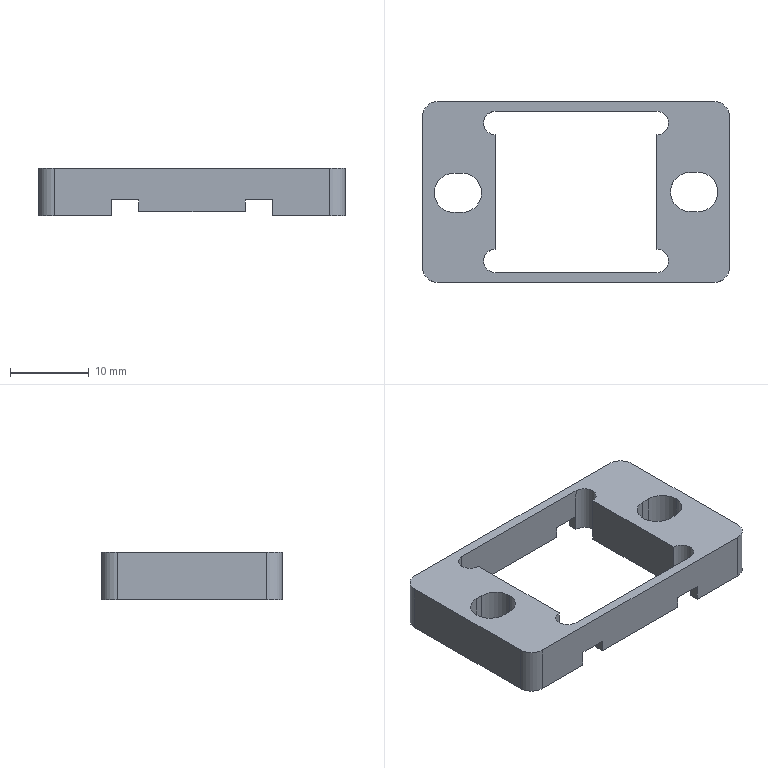Part | SolidWorks | features ICE 4, Cut 1, Extrusion 1, Fillet 1 | 1 solid | 45 faces | box 39 x 23 x 6 mm | volume 2408 mm3 | plane 29 | cylinder 16 | commonest cylinder face diameters 3 x6 5 x6 4 x4
STEP:
#1=CARTESIAN_POINT('',(-12.,-0.1,0.));
#2=VERTEX_POINT('',#1);
#3=CARTESIAN_POINT('',(-14.5,2.4,0.));
#4=VERTEX_POINT('',#3);
#5=CARTESIAN_POINT('',(-14.5,-0.1,0.));
#6=DIRECTION('',(0.,0.,1.));
#7=DIRECTION('',(1.,0.,0.));
#8=AXIS2_PLACEMENT_3D('',#5,#6,#7);
#9=CIRCLE('',#8,2.5);
#10=EDGE_CURVE('',#2,#4,#9,.T.);
#11=ORIENTED_EDGE('',*,*,#10,.F.);
#12=CARTESIAN_POINT('',(-12.,-0.1,6.));
#13=VERTEX_POINT('',#12);
#14=CARTESIAN_POINT('',(-12.,-0.1,-4.));
#15=DIRECTION('',(0.,0.,1.));
#16=VECTOR('',#15,1000.);
#17=LINE('',#14,#16);
#18=EDGE_CURVE('',#2,#13,#17,.T.);
#19=ORIENTED_EDGE('',*,*,#18,.T.);
#20=CARTESIAN_POINT('',(-14.5,2.4,6.));
#21=VERTEX_POINT('',#20);
#22=CARTESIAN_POINT('',(-14.5,-0.1,6.));
#23=DIRECTION('',(0.,0.,1.));
#24=DIRECTION('',(1.,0.,0.));
#25=AXIS2_PLACEMENT_3D('',#22,#23,#24);
#26=CIRCLE('',#25,2.5);
#27=EDGE_CURVE('',#13,#21,#26,.T.);
#28=ORIENTED_EDGE('',*,*,#27,.T.);
#29=CARTESIAN_POINT('',(-14.5,2.4,-4.));
#30=DIRECTION('',(0.,0.,1.));
#31=VECTOR('',#30,1000.);
#32=LINE('',#29,#31);
#33=EDGE_CURVE('',#4,#21,#32,.T.);
#34=ORIENTED_EDGE('',*,*,#33,.F.);
#35=EDGE_LOOP('',(#11,#19,#28,#34));
#36=FACE_OUTER_BOUND('',#35,.T.);
#37=CARTESIAN_POINT('',(-14.5,-0.1,-4.));
#38=DIRECTION('',(0.,0.,1.));
#39=DIRECTION('',(1.,0.,0.));
#40=AXIS2_PLACEMENT_3D('',#37,#38,#39);
#41=CYLINDRICAL_SURFACE('',#40,2.5);
#42=ADVANCED_FACE('',(#36),#41,.F.);
#43=CARTESIAN_POINT('',(18.,0.,0.));
#44=VERTEX_POINT('',#43);
#45=CARTESIAN_POINT('',(15.5,2.5,0.));
#46=VERTEX_POINT('',#45);
#47=CARTESIAN_POINT('',(15.5,0.,0.));
#48=DIRECTION('',(0.,0.,1.));
#49=DIRECTION('',(1.,0.,0.));
#50=AXIS2_PLACEMENT_3D('',#47,#48,#49);
#51=CIRCLE('',#50,2.5);
#52=EDGE_CURVE('',#44,#46,#51,.T.);
#53=ORIENTED_EDGE('',*,*,#52,.F.);
#54=CARTESIAN_POINT('',(18.,0.,6.));
#55=VERTEX_POINT('',#54);
#56=CARTESIAN_POINT('',(18.,0.,-4.));
#57=DIRECTION('',(0.,0.,1.));
#58=VECTOR('',#57,1000.);
#59=LINE('',#56,#58);
#60=EDGE_CURVE('',#44,#55,#59,.T.);
#61=ORIENTED_EDGE('',*,*,#60,.T.);
#62=CARTESIAN_POINT('',(15.5,2.5,6.));
#63=VERTEX_POINT('',#62);
#64=CARTESIAN_POINT('',(15.5,0.,6.));
#65=DIRECTION('',(0.,0.,1.));
#66=DIRECTION('',(1.,0.,0.));
#67=AXIS2_PLACEMENT_3D('',#64,#65,#66);
#68=CIRCLE('',#67,2.5);
#69=EDGE_CURVE('',#55,#63,#68,.T.);
#70=ORIENTED_EDGE('',*,*,#69,.T.);
#71=CARTESIAN_POINT('',(15.5,2.5,-4.));
#72=DIRECTION('',(0.,0.,1.));
#73=VECTOR('',#72,1000.);
#74=LINE('',#71,#73);
#75=EDGE_CURVE('',#46,#63,#74,.T.);
#76=ORIENTED_EDGE('',*,*,#75,.F.);
#77=EDGE_LOOP('',(#53,#61,#70,#76));
#78=FACE_OUTER_BOUND('',#77,.T.);
#79=CARTESIAN_POINT('',(15.5,0.,-4.));
#80=DIRECTION('',(0.,0.,1.));
#81=DIRECTION('',(1.,0.,0.));
#82=AXIS2_PLACEMENT_3D('',#79,#80,#81);
#83=CYLINDRICAL_SURFACE('',#82,2.5);
#84=ADVANCED_FACE('',(#78),#83,.F.);
#85=CARTESIAN_POINT('',(-11.75,8.75,6.));
#86=VERTEX_POINT('',#85);
#87=CARTESIAN_POINT('',(-10.25,10.25,6.));
#88=VERTEX_POINT('',#87);
#89=CARTESIAN_POINT('',(-10.25,8.75,6.));
#90=DIRECTION('',(0.,0.,-1.));
#91=DIRECTION('',(1.,0.,0.));
#92=AXIS2_PLACEMENT_3D('',#89,#90,#91);
#93=CIRCLE('',#92,1.5);
#94=EDGE_CURVE('',#86,#88,#93,.T.);
#95=ORIENTED_EDGE('',*,*,#94,.F.);
#96=CARTESIAN_POINT('',(-11.75,8.75,0.));
#97=VERTEX_POINT('',#96);
#98=CARTESIAN_POINT('',(-11.75,8.75,29.691));
#99=DIRECTION('',(0.,0.,-1.));
#100=VECTOR('',#99,1000.);
#101=LINE('',#98,#100);
#102=EDGE_CURVE('',#86,#97,#101,.T.);
#103=ORIENTED_EDGE('',*,*,#102,.T.);
#104=CARTESIAN_POINT('',(-10.25,10.25,0.));
#105=VERTEX_POINT('',#104);
#106=CARTESIAN_POINT('',(-10.25,8.75,0.));
#107=DIRECTION('',(0.,0.,-1.));
#108=DIRECTION('',(-1.,0.,0.));
#109=AXIS2_PLACEMENT_3D('',#106,#107,#108);
#110=CIRCLE('',#109,1.5);
#111=EDGE_CURVE('',#97,#105,#110,.T.);
#112=ORIENTED_EDGE('',*,*,#111,.T.);
#113=CARTESIAN_POINT('',(-10.25,10.25,2.));
#114=VERTEX_POINT('',#113);
#115=CARTESIAN_POINT('',(-10.25,10.25,29.691));
#116=DIRECTION('',(0.,0.,-1.));
#117=VECTOR('',#116,1000.);
#118=LINE('',#115,#117);
#119=EDGE_CURVE('',#114,#105,#118,.T.);
#120=ORIENTED_EDGE('',*,*,#119,.F.);
#121=CARTESIAN_POINT('',(-10.25,10.25,6.));
#122=DIRECTION('',(0.,0.,-1.));
#123=VECTOR('',#122,1000.);
#124=LINE('',#121,#123);
#125=EDGE_CURVE('',#88,#114,#124,.T.);
#126=ORIENTED_EDGE('',*,*,#125,.F.);
#127=EDGE_LOOP('',(#95,#103,#112,#120,#126));
#128=FACE_OUTER_BOUND('',#127,.T.);
#129=CARTESIAN_POINT('',(-10.25,8.75,29.691));
#130=DIRECTION('',(0.,0.,-1.));
#131=DIRECTION('',(-1.,0.,0.));
#132=AXIS2_PLACEMENT_3D('',#129,#130,#131);
#133=CYLINDRICAL_SURFACE('',#132,1.5);
#134=ADVANCED_FACE('',(#128),#133,.F.);
#135=CARTESIAN_POINT('',(-11.75,-8.75,6.));
#136=VERTEX_POINT('',#135);
#137=CARTESIAN_POINT('',(-10.25,-7.25,6.));
#138=VERTEX_POINT('',#137);
#139=CARTESIAN_POINT('',(-10.25,-8.75,6.));
#140=DIRECTION('',(0.,0.,-1.));
#141=DIRECTION('',(1.,0.,0.));
#142=AXIS2_PLACEMENT_3D('',#139,#140,#141);
#143=CIRCLE('',#142,1.5);
#144=EDGE_CURVE('',#136,#138,#143,.T.);
#145=ORIENTED_EDGE('',*,*,#144,.F.);
#146=CARTESIAN_POINT('',(-11.75,-8.75,0.));
#147=VERTEX_POINT('',#146);
#148=CARTESIAN_POINT('',(-11.75,-8.75,29.691));
#149=DIRECTION('',(0.,0.,-1.));
#150=VECTOR('',#149,1000.);
#151=LINE('',#148,#150);
#152=EDGE_CURVE('',#136,#147,#151,.T.);
#153=ORIENTED_EDGE('',*,*,#152,.T.);
#154=CARTESIAN_POINT('',(-10.25,-7.25,0.));
#155=VERTEX_POINT('',#154);
#156=CARTESIAN_POINT('',(-10.25,-8.75,0.));
#157=DIRECTION('',(0.,0.,-1.));
#158=DIRECTION('',(-1.,0.,0.));
#159=AXIS2_PLACEMENT_3D('',#156,#157,#158);
#160=CIRCLE('',#159,1.5);
#161=EDGE_CURVE('',#147,#155,#160,.T.);
#162=ORIENTED_EDGE('',*,*,#161,.T.);
#163=CARTESIAN_POINT('',(-10.25,-7.25,29.691));
#164=DIRECTION('',(0.,0.,-1.));
#165=VECTOR('',#164,1000.);
#166=LINE('',#163,#165);
#167=EDGE_CURVE('',#138,#155,#166,.T.);
#168=ORIENTED_EDGE('',*,*,#167,.F.);
#169=EDGE_LOOP('',(#145,#153,#162,#168));
#170=FACE_OUTER_BOUND('',#169,.T.);
#171=CARTESIAN_POINT('',(-10.25,-8.75,29.691));
#172=DIRECTION('',(0.,0.,-1.));
#173=DIRECTION('',(-1.,0.,0.));
#174=AXIS2_PLACEMENT_3D('',#171,#172,#173);
#175=CYLINDRICAL_SURFACE('',#174,1.5);
#176=ADVANCED_FACE('',(#170),#175,.F.);
#177=CARTESIAN_POINT('',(10.25,10.25,2.));
#178=VERTEX_POINT('',#177);
#179=CARTESIAN_POINT('',(10.25,10.25,0.));
#180=VERTEX_POINT('',#179);
#181=CARTESIAN_POINT('',(10.25,10.25,29.691));
#182=DIRECTION('',(0.,0.,-1.));
#183=VECTOR('',#182,1000.);
#184=LINE('',#181,#183);
#185=EDGE_CURVE('',#178,#180,#184,.T.);
#186=ORIENTED_EDGE('',*,*,#185,.F.);
#187=CARTESIAN_POINT('',(10.25,11.5,2.));
#188=VERTEX_POINT('',#187);
#189=CARTESIAN_POINT('',(10.25,32.097,2.));
#190=DIRECTION('',(0.,-1.,0.));
#191=VECTOR('',#190,1000.);
#192=LINE('',#189,#191);
#193=EDGE_CURVE('',#188,#178,#192,.T.);
#194=ORIENTED_EDGE('',*,*,#193,.F.);
#195=CARTESIAN_POINT('',(10.25,11.5,0.));
#196=VERTEX_POINT('',#195);
#197=CARTESIAN_POINT('',(10.25,11.5,0.));
#198=DIRECTION('',(0.,0.,-1.));
#199=VECTOR('',#198,1000.);
#200=LINE('',#197,#199);
#201=EDGE_CURVE('',#188,#196,#200,.T.);
#202=ORIENTED_EDGE('',*,*,#201,.T.);
#203=CARTESIAN_POINT('',(10.25,10.25,0.));
#204=DIRECTION('',(0.,1.,0.));
#205=VECTOR('',#204,1000.);
#206=LINE('',#203,#205);
#207=EDGE_CURVE('',#180,#196,#206,.T.);
#208=ORIENTED_EDGE('',*,*,#207,.F.);
#209=EDGE_LOOP('',(#186,#194,#202,#208));
#210=FACE_OUTER_BOUND('',#209,.T.);
#211=CARTESIAN_POINT('',(10.25,10.25,6.));
#212=DIRECTION('',(-1.,0.,0.));
#213=DIRECTION('',(0.,-1.,0.));
#214=AXIS2_PLACEMENT_3D('',#211,#212,#213);
#215=PLANE('',#214);
#216=ADVANCED_FACE('',(#210),#215,.T.);
#217=CARTESIAN_POINT('',(10.25,7.25,6.));
#218=VERTEX_POINT('',#217);
#219=CARTESIAN_POINT('',(10.25,7.25,0.));
#220=VERTEX_POINT('',#219);
#221=CARTESIAN_POINT('',(10.25,7.25,29.691));
#222=DIRECTION('',(0.,0.,-1.));
#223=VECTOR('',#222,1000.);
#224=LINE('',#221,#223);
#225=EDGE_CURVE('',#218,#220,#224,.T.);
#226=ORIENTED_EDGE('',*,*,#225,.T.);
#227=CARTESIAN_POINT('',(10.25,-7.25,0.));
#228=VERTEX_POINT('',#227);
#229=CARTESIAN_POINT('',(10.25,10.25,0.));
#230=DIRECTION('',(0.,1.,0.));
#231=VECTOR('',#230,1000.);
#232=LINE('',#229,#231);
#233=EDGE_CURVE('',#228,#220,#232,.T.);
#234=ORIENTED_EDGE('',*,*,#233,.F.);
#235=CARTESIAN_POINT('',(10.25,-7.25,6.));
#236=VERTEX_POINT('',#235);
#237=CARTESIAN_POINT('',(10.25,-7.25,29.691));
#238=DIRECTION('',(0.,0.,-1.));
#239=VECTOR('',#238,1000.);
#240=LINE('',#237,#239);
#241=EDGE_CURVE('',#236,#228,#240,.T.);
#242=ORIENTED_EDGE('',*,*,#241,.F.);
#243=CARTESIAN_POINT('',(10.25,10.25,6.));
#244=DIRECTION('',(0.,1.,0.));
#245=VECTOR('',#244,1000.);
#246=LINE('',#243,#245);
#247=EDGE_CURVE('',#236,#218,#246,.T.);
#248=ORIENTED_EDGE('',*,*,#247,.T.);
#249=EDGE_LOOP('',(#226,#234,#242,#248));
#250=FACE_OUTER_BOUND('',#249,.T.);
#251=CARTESIAN_POINT('',(10.25,10.25,6.));
#252=DIRECTION('',(-1.,0.,0.));
#253=DIRECTION('',(0.,-1.,0.));
#254=AXIS2_PLACEMENT_3D('',#251,#252,#253);
#255=PLANE('',#254);
#256=ADVANCED_FACE('',(#250),#255,.T.);
#257=CARTESIAN_POINT('',(-10.25,7.25,6.));
#258=VERTEX_POINT('',#257);
#259=CARTESIAN_POINT('',(-10.25,7.25,0.));
#260=VERTEX_POINT('',#259);
#261=CARTESIAN_POINT('',(-10.25,7.25,29.691));
#262=DIRECTION('',(0.,0.,-1.));
#263=VECTOR('',#262,1000.);
#264=LINE('',#261,#263);
#265=EDGE_CURVE('',#258,#260,#264,.T.);
#266=ORIENTED_EDGE('',*,*,#265,.F.);
#267=CARTESIAN_POINT('',(-10.25,10.25,6.));
#268=DIRECTION('',(0.,-1.,0.));
#269=VECTOR('',#268,1000.);
#270=LINE('',#267,#269);
#271=EDGE_CURVE('',#258,#138,#270,.T.);
#272=ORIENTED_EDGE('',*,*,#271,.T.);
#273=ORIENTED_EDGE('',*,*,#167,.T.);
#274=CARTESIAN_POINT('',(-10.25,10.25,0.));
#275=DIRECTION('',(0.,-1.,0.));
#276=VECTOR('',#275,1000.);
#277=LINE('',#274,#276);
#278=EDGE_CURVE('',#260,#155,#277,.T.);
#279=ORIENTED_EDGE('',*,*,#278,.F.);
#280=EDGE_LOOP('',(#266,#272,#273,#279));
#281=FACE_OUTER_BOUND('',#280,.T.);
#282=CARTESIAN_POINT('',(-10.25,10.25,6.));
#283=DIRECTION('',(1.,0.,0.));
#284=DIRECTION('',(0.,1.,0.));
#285=AXIS2_PLACEMENT_3D('',#282,#283,#284);
#286=PLANE('',#285);
#287=ADVANCED_FACE('',(#281),#286,.T.);
#288=CARTESIAN_POINT('',(-10.25,-10.25,2.));
#289=VERTEX_POINT('',#288);
#290=CARTESIAN_POINT('',(-10.25,-10.25,0.));
#291=VERTEX_POINT('',#290);
#292=CARTESIAN_POINT('',(-10.25,-10.25,29.691));
#293=DIRECTION('',(0.,0.,-1.));
#294=VECTOR('',#293,1000.);
#295=LINE('',#292,#294);
#296=EDGE_CURVE('',#289,#291,#295,.T.);
#297=ORIENTED_EDGE('',*,*,#296,.F.);
#298=CARTESIAN_POINT('',(-10.25,-11.5,2.));
#299=VERTEX_POINT('',#298);
#300=CARTESIAN_POINT('',(-10.25,32.097,2.));
#301=DIRECTION('',(0.,-1.,0.));
#302=VECTOR('',#301,1000.);
#303=LINE('',#300,#302);
#304=EDGE_CURVE('',#289,#299,#303,.T.);
#305=ORIENTED_EDGE('',*,*,#304,.T.);
#306=CARTESIAN_POINT('',(-10.25,-11.5,0.));
#307=VERTEX_POINT('',#306);
#308=CARTESIAN_POINT('',(-10.25,-11.5,0.));
#309=DIRECTION('',(0.,0.,-1.));
#310=VECTOR('',#309,1000.);
#311=LINE('',#308,#310);
#312=EDGE_CURVE('',#299,#307,#311,.T.);
#313=ORIENTED_EDGE('',*,*,#312,.T.);
#314=CARTESIAN_POINT('',(-10.25,10.25,0.));
#315=DIRECTION('',(0.,-1.,0.));
#316=VECTOR('',#315,1000.);
#317=LINE('',#314,#316);
#318=EDGE_CURVE('',#291,#307,#317,.T.);
#319=ORIENTED_EDGE('',*,*,#318,.F.);
#320=EDGE_LOOP('',(#297,#305,#313,#319));
#321=FACE_OUTER_BOUND('',#320,.T.);
#322=CARTESIAN_POINT('',(-10.25,10.25,6.));
#323=DIRECTION('',(1.,0.,0.));
#324=DIRECTION('',(0.,1.,0.));
#325=AXIS2_PLACEMENT_3D('',#322,#323,#324);
#326=PLANE('',#325);
#327=ADVANCED_FACE('',(#321),#326,.T.);
#328=CARTESIAN_POINT('',(-15.5,2.4,0.));
#329=VERTEX_POINT('',#328);
#330=CARTESIAN_POINT('',(0.,2.4,0.));
#331=DIRECTION('',(-1.,0.,0.));
#332=VECTOR('',#331,1000.);
#333=LINE('',#330,#332);
#334=EDGE_CURVE('',#4,#329,#333,.T.);
#335=ORIENTED_EDGE('',*,*,#334,.T.);
#336=CARTESIAN_POINT('',(-15.5,-2.6,0.));
#337=VERTEX_POINT('',#336);
#338=CARTESIAN_POINT('',(-15.5,-0.1,0.));
#339=DIRECTION('',(0.,0.,1.));
#340=DIRECTION('',(1.,0.,0.));
#341=AXIS2_PLACEMENT_3D('',#338,#339,#340);
#342=CIRCLE('',#341,2.5);
#343=EDGE_CURVE('',#329,#337,#342,.T.);
#344=ORIENTED_EDGE('',*,*,#343,.T.);
#345=CARTESIAN_POINT('',(-14.5,-2.6,0.));
#346=VERTEX_POINT('',#345);
#347=CARTESIAN_POINT('',(0.,-2.6,0.));
#348=DIRECTION('',(1.,0.,0.));
#349=VECTOR('',#348,1000.);
#350=LINE('',#347,#349);
#351=EDGE_CURVE('',#337,#346,#350,.T.);
#352=ORIENTED_EDGE('',*,*,#351,.T.);
#353=CARTESIAN_POINT('',(-14.5,-0.1,0.));
#354=DIRECTION('',(0.,0.,1.));
#355=DIRECTION('',(1.,0.,0.));
#356=AXIS2_PLACEMENT_3D('',#353,#354,#355);
#357=CIRCLE('',#356,2.5);
#358=EDGE_CURVE('',#346,#2,#357,.T.);
#359=ORIENTED_EDGE('',*,*,#358,.T.);
#360=ORIENTED_EDGE('',*,*,#10,.T.);
#361=EDGE_LOOP('',(#335,#344,#352,#359,#360));
#362=FACE_BOUND('',#361,.T.);
#363=CARTESIAN_POINT('',(-19.5,9.5,0.));
#364=VERTEX_POINT('',#363);
#365=CARTESIAN_POINT('',(-19.5,-9.5,0.));
#366=VERTEX_POINT('',#365);
#367=CARTESIAN_POINT('',(-19.5,11.5,0.));
#368=DIRECTION('',(0.,-1.,0.));
#369=VECTOR('',#368,1000.);
#370=LINE('',#367,#369);
#371=EDGE_CURVE('',#364,#366,#370,.T.);
#372=ORIENTED_EDGE('',*,*,#371,.F.);
#373=CARTESIAN_POINT('',(-17.5,11.5,0.));
#374=VERTEX_POINT('',#373);
#375=CARTESIAN_POINT('',(-17.5,9.5,0.));
#376=DIRECTION('',(0.,0.,-1.));
#377=DIRECTION('',(1.,0.,0.));
#378=AXIS2_PLACEMENT_3D('',#375,#376,#377);
#379=CIRCLE('',#378,2.);
#380=EDGE_CURVE('',#364,#374,#379,.T.);
#381=ORIENTED_EDGE('',*,*,#380,.T.);
#382=CARTESIAN_POINT('',(-10.25,11.5,0.));
#383=VERTEX_POINT('',#382);
#384=CARTESIAN_POINT('',(-19.5,11.5,0.));
#385=DIRECTION('',(-1.,0.,0.));
#386=VECTOR('',#385,1000.);
#387=LINE('',#384,#386);
#388=EDGE_CURVE('',#383,#374,#387,.T.);
#389=ORIENTED_EDGE('',*,*,#388,.F.);
#390=CARTESIAN_POINT('',(-10.25,10.25,0.));
#391=DIRECTION('',(0.,-1.,0.));
#392=VECTOR('',#391,1000.);
#393=LINE('',#390,#392);
#394=EDGE_CURVE('',#383,#105,#393,.T.);
#395=ORIENTED_EDGE('',*,*,#394,.T.);
#396=ORIENTED_EDGE('',*,*,#111,.F.);
#397=CARTESIAN_POINT('',(-10.25,8.75,0.));
#398=DIRECTION('',(0.,0.,-1.));
#399=DIRECTION('',(-1.,0.,0.));
#400=AXIS2_PLACEMENT_3D('',#397,#398,#399);
#401=CIRCLE('',#400,1.5);
#402=EDGE_CURVE('',#260,#97,#401,.T.);
#403=ORIENTED_EDGE('',*,*,#402,.F.);
#404=ORIENTED_EDGE('',*,*,#278,.T.);
#405=ORIENTED_EDGE('',*,*,#161,.F.);
#406=CARTESIAN_POINT('',(-10.25,-8.75,0.));
#407=DIRECTION('',(0.,0.,-1.));
#408=DIRECTION('',(-1.,0.,0.));
#409=AXIS2_PLACEMENT_3D('',#406,#407,#408);
#410=CIRCLE('',#409,1.5);
#411=EDGE_CURVE('',#291,#147,#410,.T.);
#412=ORIENTED_EDGE('',*,*,#411,.F.);
#413=ORIENTED_EDGE('',*,*,#318,.T.);
#414=CARTESIAN_POINT('',(-17.5,-11.5,0.));
#415=VERTEX_POINT('',#414);
#416=CARTESIAN_POINT('',(-19.5,-11.5,0.));
#417=DIRECTION('',(1.,0.,0.));
#418=VECTOR('',#417,1000.);
#419=LINE('',#416,#418);
#420=EDGE_CURVE('',#415,#307,#419,.T.);
#421=ORIENTED_EDGE('',*,*,#420,.F.);
#422=CARTESIAN_POINT('',(-17.5,-9.5,0.));
#423=DIRECTION('',(0.,0.,-1.));
#424=DIRECTION('',(1.,0.,0.));
#425=AXIS2_PLACEMENT_3D('',#422,#423,#424);
#426=CIRCLE('',#425,2.);
#427=EDGE_CURVE('',#415,#366,#426,.T.);
#428=ORIENTED_EDGE('',*,*,#427,.T.);
#429=EDGE_LOOP('',(#372,#381,#389,#395,#396,#403,#404,#405,#412,#413,#421,#428));
#430=FACE_OUTER_BOUND('',#429,.T.);
#431=CARTESIAN_POINT('',(0.,0.,0.));
#432=DIRECTION('',(0.,0.,1.));
#433=DIRECTION('',(1.,0.,0.));
#434=AXIS2_PLACEMENT_3D('',#431,#432,#433);
#435=PLANE('',#434);
#436=ADVANCED_FACE('',(#362,#430),#435,.F.);
#437=CARTESIAN_POINT('',(-15.5,2.4,6.));
#438=VERTEX_POINT('',#437);
#439=CARTESIAN_POINT('',(-15.5,-2.6,6.));
#440=VERTEX_POINT('',#439);
#441=CARTESIAN_POINT('',(-15.5,-0.1,6.));
#442=DIRECTION('',(0.,0.,1.));
#443=DIRECTION('',(1.,0.,0.));
#444=AXIS2_PLACEMENT_3D('',#441,#442,#443);
#445=CIRCLE('',#444,2.5);
#446=EDGE_CURVE('',#438,#440,#445,.T.);
#447=ORIENTED_EDGE('',*,*,#446,.F.);
#448=CARTESIAN_POINT('',(-15.5,2.4,6.));
#449=DIRECTION('',(-1.,0.,0.));
#450=VECTOR('',#449,1000.);
#451=LINE('',#448,#450);
#452=EDGE_CURVE('',#21,#438,#451,.T.);
#453=ORIENTED_EDGE('',*,*,#452,.F.);
#454=ORIENTED_EDGE('',*,*,#27,.F.);
#455=CARTESIAN_POINT('',(-14.5,-2.6,6.));
#456=VERTEX_POINT('',#455);
#457=CARTESIAN_POINT('',(-14.5,-0.1,6.));
#458=DIRECTION('',(0.,0.,1.));
#459=DIRECTION('',(1.,0.,0.));
#460=AXIS2_PLACEMENT_3D('',#457,#458,#459);
#461=CIRCLE('',#460,2.5);
#462=EDGE_CURVE('',#456,#13,#461,.T.);
#463=ORIENTED_EDGE('',*,*,#462,.F.);
#464=CARTESIAN_POINT('',(-15.5,-2.6,6.));
#465=DIRECTION('',(1.,0.,0.));
#466=VECTOR('',#465,1000.);
#467=LINE('',#464,#466);
#468=EDGE_CURVE('',#440,#456,#467,.T.);
#469=ORIENTED_EDGE('',*,*,#468,.F.);
#470=EDGE_LOOP('',(#447,#453,#454,#463,#469));
#471=FACE_BOUND('',#470,.T.);
#472=CARTESIAN_POINT('',(14.5,2.5,6.));
#473=VERTEX_POINT('',#472);
#474=CARTESIAN_POINT('',(14.5,-2.5,6.));
#475=VERTEX_POINT('',#474);
#476=CARTESIAN_POINT('',(14.5,0.,6.));
#477=DIRECTION('',(0.,0.,1.));
#478=DIRECTION('',(1.,0.,0.));
#479=AXIS2_PLACEMENT_3D('',#476,#477,#478);
#480=CIRCLE('',#479,2.5);
#481=EDGE_CURVE('',#473,#475,#480,.T.);
#482=ORIENTED_EDGE('',*,*,#481,.F.);
#483=CARTESIAN_POINT('',(14.5,2.5,6.));
#484=DIRECTION('',(-1.,0.,0.));
#485=VECTOR('',#484,1000.);
#486=LINE('',#483,#485);
#487=EDGE_CURVE('',#63,#473,#486,.T.);
#488=ORIENTED_EDGE('',*,*,#487,.F.);
#489=ORIENTED_EDGE('',*,*,#69,.F.);
#490=CARTESIAN_POINT('',(15.5,-2.5,6.));
#491=VERTEX_POINT('',#490);
#492=CARTESIAN_POINT('',(15.5,0.,6.));
#493=DIRECTION('',(0.,0.,1.));
#494=DIRECTION('',(1.,0.,0.));
#495=AXIS2_PLACEMENT_3D('',#492,#493,#494);
#496=CIRCLE('',#495,2.5);
#497=EDGE_CURVE('',#491,#55,#496,.T.);
#498=ORIENTED_EDGE('',*,*,#497,.F.);
#499=CARTESIAN_POINT('',(14.5,-2.5,6.));
#500=DIRECTION('',(1.,0.,0.));
#501=VECTOR('',#500,1000.);
#502=LINE('',#499,#501);
#503=EDGE_CURVE('',#475,#491,#502,.T.);
#504=ORIENTED_EDGE('',*,*,#503,.F.);
#505=EDGE_LOOP('',(#482,#488,#489,#498,#504));
#506=FACE_BOUND('',#505,.T.);
#507=CARTESIAN_POINT('',(-10.25,8.75,6.));
#508=DIRECTION('',(0.,0.,-1.));
#509=DIRECTION('',(1.,0.,0.));
#510=AXIS2_PLACEMENT_3D('',#507,#508,#509);
#511=CIRCLE('',#510,1.5);
#512=EDGE_CURVE('',#258,#86,#511,.T.);
#513=ORIENTED_EDGE('',*,*,#512,.T.);
#514=ORIENTED_EDGE('',*,*,#94,.T.);
#515=CARTESIAN_POINT('',(10.25,10.25,6.));
#516=VERTEX_POINT('',#515);
#517=CARTESIAN_POINT('',(-10.25,10.25,6.));
#518=DIRECTION('',(1.,0.,0.));
#519=VECTOR('',#518,1000.);
#520=LINE('',#517,#519);
#521=EDGE_CURVE('',#88,#516,#520,.T.);
#522=ORIENTED_EDGE('',*,*,#521,.T.);
#523=CARTESIAN_POINT('',(10.25,8.75,6.));
#524=DIRECTION('',(0.,0.,-1.));
#525=DIRECTION('',(1.,0.,0.));
#526=AXIS2_PLACEMENT_3D('',#523,#524,#525);
#527=CIRCLE('',#526,1.5);
#528=EDGE_CURVE('',#516,#218,#527,.T.);
#529=ORIENTED_EDGE('',*,*,#528,.T.);
#530=ORIENTED_EDGE('',*,*,#247,.F.);
#531=CARTESIAN_POINT('',(10.25,-10.25,6.));
#532=VERTEX_POINT('',#531);
#533=CARTESIAN_POINT('',(10.25,-8.75,6.));
#534=DIRECTION('',(0.,0.,-1.));
#535=DIRECTION('',(1.,0.,0.));
#536=AXIS2_PLACEMENT_3D('',#533,#534,#535);
#537=CIRCLE('',#536,1.5);
#538=EDGE_CURVE('',#236,#532,#537,.T.);
#539=ORIENTED_EDGE('',*,*,#538,.T.);
#540=CARTESIAN_POINT('',(-10.25,-10.25,6.));
#541=VERTEX_POINT('',#540);
#542=CARTESIAN_POINT('',(-10.25,-10.25,6.));
#543=DIRECTION('',(-1.,0.,0.));
#544=VECTOR('',#543,1000.);
#545=LINE('',#542,#544);
#546=EDGE_CURVE('',#532,#541,#545,.T.);
#547=ORIENTED_EDGE('',*,*,#546,.T.);
#548=CARTESIAN_POINT('',(-10.25,-8.75,6.));
#549=DIRECTION('',(0.,0.,-1.));
#550=DIRECTION('',(1.,0.,0.));
#551=AXIS2_PLACEMENT_3D('',#548,#549,#550);
#552=CIRCLE('',#551,1.5);
#553=EDGE_CURVE('',#541,#136,#552,.T.);
#554=ORIENTED_EDGE('',*,*,#553,.T.);
#555=ORIENTED_EDGE('',*,*,#144,.T.);
#556=ORIENTED_EDGE('',*,*,#271,.F.);
#557=EDGE_LOOP('',(#513,#514,#522,#529,#530,#539,#547,#554,#555,#556));
#558=FACE_BOUND('',#557,.T.);
#559=CARTESIAN_POINT('',(17.5,11.5,6.));
#560=VERTEX_POINT('',#559);
#561=CARTESIAN_POINT('',(-17.5,11.5,6.));
#562=VERTEX_POINT('',#561);
#563=CARTESIAN_POINT('',(-19.5,11.5,6.));
#564=DIRECTION('',(-1.,0.,0.));
#565=VECTOR('',#564,1000.);
#566=LINE('',#563,#565);
#567=EDGE_CURVE('',#560,#562,#566,.T.);
#568=ORIENTED_EDGE('',*,*,#567,.T.);
#569=CARTESIAN_POINT('',(-19.5,9.5,6.));
#570=VERTEX_POINT('',#569);
#571=CARTESIAN_POINT('',(-17.5,9.5,6.));
#572=DIRECTION('',(0.,0.,1.));
#573=DIRECTION('',(1.,0.,0.));
#574=AXIS2_PLACEMENT_3D('',#571,#572,#573);
#575=CIRCLE('',#574,2.);
#576=EDGE_CURVE('',#562,#570,#575,.T.);
#577=ORIENTED_EDGE('',*,*,#576,.T.);
#578=CARTESIAN_POINT('',(-19.5,-9.5,6.));
#579=VERTEX_POINT('',#578);
#580=CARTESIAN_POINT('',(-19.5,11.5,6.));
#581=DIRECTION('',(0.,-1.,0.));
#582=VECTOR('',#581,1000.);
#583=LINE('',#580,#582);
#584=EDGE_CURVE('',#570,#579,#583,.T.);
#585=ORIENTED_EDGE('',*,*,#584,.T.);
#586=CARTESIAN_POINT('',(-17.5,-11.5,6.));
#587=VERTEX_POINT('',#586);
#588=CARTESIAN_POINT('',(-17.5,-9.5,6.));
#589=DIRECTION('',(0.,0.,1.));
#590=DIRECTION('',(1.,0.,0.));
#591=AXIS2_PLACEMENT_3D('',#588,#589,#590);
#592=CIRCLE('',#591,2.);
#593=EDGE_CURVE('',#579,#587,#592,.T.);
#594=ORIENTED_EDGE('',*,*,#593,.T.);
#595=CARTESIAN_POINT('',(17.5,-11.5,6.));
#596=VERTEX_POINT('',#595);
#597=CARTESIAN_POINT('',(-19.5,-11.5,6.));
#598=DIRECTION('',(1.,0.,0.));
#599=VECTOR('',#598,1000.);
#600=LINE('',#597,#599);
#601=EDGE_CURVE('',#587,#596,#600,.T.);
#602=ORIENTED_EDGE('',*,*,#601,.T.);
#603=CARTESIAN_POINT('',(19.5,-9.5,6.));
#604=VERTEX_POINT('',#603);
#605=CARTESIAN_POINT('',(17.5,-9.5,6.));
#606=DIRECTION('',(0.,0.,1.));
#607=DIRECTION('',(1.,0.,0.));
#608=AXIS2_PLACEMENT_3D('',#605,#606,#607);
#609=CIRCLE('',#608,2.);
#610=EDGE_CURVE('',#596,#604,#609,.T.);
#611=ORIENTED_EDGE('',*,*,#610,.T.);
#612=CARTESIAN_POINT('',(19.5,9.5,6.));
#613=VERTEX_POINT('',#612);
#614=CARTESIAN_POINT('',(19.5,11.5,6.));
#615=DIRECTION('',(0.,1.,0.));
#616=VECTOR('',#615,1000.);
#617=LINE('',#614,#616);
#618=EDGE_CURVE('',#604,#613,#617,.T.);
#619=ORIENTED_EDGE('',*,*,#618,.T.);
#620=CARTESIAN_POINT('',(17.5,9.5,6.));
#621=DIRECTION('',(0.,0.,1.));
#622=DIRECTION('',(1.,0.,0.));
#623=AXIS2_PLACEMENT_3D('',#620,#621,#622);
#624=CIRCLE('',#623,2.);
#625=EDGE_CURVE('',#613,#560,#624,.T.);
#626=ORIENTED_EDGE('',*,*,#625,.T.);
#627=EDGE_LOOP('',(#568,#577,#585,#594,#602,#611,#619,#626));
#628=FACE_OUTER_BOUND('',#627,.T.);
#629=CARTESIAN_POINT('',(0.,0.,6.));
#630=DIRECTION('',(0.,0.,1.));
#631=DIRECTION('',(1.,0.,0.));
#632=AXIS2_PLACEMENT_3D('',#629,#630,#631);
#633=PLANE('',#632);
#634=ADVANCED_FACE('',(#471,#506,#558,#628),#633,.T.);
#635=CARTESIAN_POINT('',(14.5,2.5,0.));
#636=VERTEX_POINT('',#635);
#637=CARTESIAN_POINT('',(0.,2.5,0.));
#638=DIRECTION('',(-1.,0.,0.));
#639=VECTOR('',#638,1000.);
#640=LINE('',#637,#639);
#641=EDGE_CURVE('',#46,#636,#640,.T.);
#642=ORIENTED_EDGE('',*,*,#641,.T.);
#643=CARTESIAN_POINT('',(14.5,-2.5,0.));
#644=VERTEX_POINT('',#643);
#645=CARTESIAN_POINT('',(14.5,0.,0.));
#646=DIRECTION('',(0.,0.,1.));
#647=DIRECTION('',(1.,0.,0.));
#648=AXIS2_PLACEMENT_3D('',#645,#646,#647);
#649=CIRCLE('',#648,2.5);
#650=EDGE_CURVE('',#636,#644,#649,.T.);
#651=ORIENTED_EDGE('',*,*,#650,.T.);
#652=CARTESIAN_POINT('',(15.5,-2.5,0.));
#653=VERTEX_POINT('',#652);
#654=CARTESIAN_POINT('',(0.,-2.5,0.));
#655=DIRECTION('',(1.,0.,0.));
#656=VECTOR('',#655,1000.);
#657=LINE('',#654,#656);
#658=EDGE_CURVE('',#644,#653,#657,.T.);
#659=ORIENTED_EDGE('',*,*,#658,.T.);
#660=CARTESIAN_POINT('',(15.5,0.,0.));
#661=DIRECTION('',(0.,0.,1.));
#662=DIRECTION('',(1.,0.,0.));
#663=AXIS2_PLACEMENT_3D('',#660,#661,#662);
#664=CIRCLE('',#663,2.5);
#665=EDGE_CURVE('',#653,#44,#664,.T.);
#666=ORIENTED_EDGE('',*,*,#665,.T.);
#667=ORIENTED_EDGE('',*,*,#52,.T.);
#668=EDGE_LOOP('',(#642,#651,#659,#666,#667));
#669=FACE_BOUND('',#668,.T.);
#670=CARTESIAN_POINT('',(19.5,-9.5,0.));
#671=VERTEX_POINT('',#670);
#672=CARTESIAN_POINT('',(19.5,9.5,0.));
#673=VERTEX_POINT('',#672);
#674=CARTESIAN_POINT('',(19.5,11.5,0.));
#675=DIRECTION('',(0.,1.,0.));
#676=VECTOR('',#675,1000.);
#677=LINE('',#674,#676);
#678=EDGE_CURVE('',#671,#673,#677,.T.);
#679=ORIENTED_EDGE('',*,*,#678,.F.);
#680=CARTESIAN_POINT('',(17.5,-11.5,0.));
#681=VERTEX_POINT('',#680);
#682=CARTESIAN_POINT('',(17.5,-9.5,0.));
#683=DIRECTION('',(0.,0.,-1.));
#684=DIRECTION('',(1.,0.,0.));
#685=AXIS2_PLACEMENT_3D('',#682,#683,#684);
#686=CIRCLE('',#685,2.);
#687=EDGE_CURVE('',#671,#681,#686,.T.);
#688=ORIENTED_EDGE('',*,*,#687,.T.);
#689=CARTESIAN_POINT('',(10.25,-11.5,0.));
#690=VERTEX_POINT('',#689);
#691=CARTESIAN_POINT('',(-19.5,-11.5,0.));
#692=DIRECTION('',(1.,0.,0.));
#693=VECTOR('',#692,1000.);
#694=LINE('',#691,#693);
#695=EDGE_CURVE('',#690,#681,#694,.T.);
#696=ORIENTED_EDGE('',*,*,#695,.F.);
#697=CARTESIAN_POINT('',(10.25,-10.25,0.));
#698=VERTEX_POINT('',#697);
#699=CARTESIAN_POINT('',(10.25,10.25,0.));
#700=DIRECTION('',(0.,1.,0.));
#701=VECTOR('',#700,1000.);
#702=LINE('',#699,#701);
#703=EDGE_CURVE('',#690,#698,#702,.T.);
#704=ORIENTED_EDGE('',*,*,#703,.T.);
#705=CARTESIAN_POINT('',(10.25,-8.75,0.));
#706=DIRECTION('',(0.,0.,-1.));
#707=DIRECTION('',(-1.,0.,0.));
#708=AXIS2_PLACEMENT_3D('',#705,#706,#707);
#709=CIRCLE('',#708,1.5);
#710=EDGE_CURVE('',#228,#698,#709,.T.);
#711=ORIENTED_EDGE('',*,*,#710,.F.);
#712=ORIENTED_EDGE('',*,*,#233,.T.);
#713=CARTESIAN_POINT('',(10.25,8.75,0.));
#714=DIRECTION('',(0.,0.,-1.));
#715=DIRECTION('',(-1.,0.,0.));
#716=AXIS2_PLACEMENT_3D('',#713,#714,#715);
#717=CIRCLE('',#716,1.5);
#718=EDGE_CURVE('',#180,#220,#717,.T.);
#719=ORIENTED_EDGE('',*,*,#718,.F.);
#720=ORIENTED_EDGE('',*,*,#207,.T.);
#721=CARTESIAN_POINT('',(17.5,11.5,0.));
#722=VERTEX_POINT('',#721);
#723=CARTESIAN_POINT('',(-19.5,11.5,0.));
#724=DIRECTION('',(-1.,0.,0.));
#725=VECTOR('',#724,1000.);
#726=LINE('',#723,#725);
#727=EDGE_CURVE('',#722,#196,#726,.T.);
#728=ORIENTED_EDGE('',*,*,#727,.F.);
#729=CARTESIAN_POINT('',(17.5,9.5,0.));
#730=DIRECTION('',(0.,0.,-1.));
#731=DIRECTION('',(1.,0.,0.));
#732=AXIS2_PLACEMENT_3D('',#729,#730,#731);
#733=CIRCLE('',#732,2.);
#734=EDGE_CURVE('',#722,#673,#733,.T.);
#735=ORIENTED_EDGE('',*,*,#734,.T.);
#736=EDGE_LOOP('',(#679,#688,#696,#704,#711,#712,#719,#720,#728,#735));
#737=FACE_OUTER_BOUND('',#736,.T.);
#738=CARTESIAN_POINT('',(0.,0.,0.));
#739=DIRECTION('',(0.,0.,1.));
#740=DIRECTION('',(1.,0.,0.));
#741=AXIS2_PLACEMENT_3D('',#738,#739,#740);
#742=PLANE('',#741);
#743=ADVANCED_FACE('',(#669,#737),#742,.F.);
#744=ORIENTED_EDGE('',*,*,#618,.F.);
#745=CARTESIAN_POINT('',(19.5,-9.5,6.));
#746=DIRECTION('',(0.,0.,-1.));
#747=VECTOR('',#746,1000.);
#748=LINE('',#745,#747);
#749=EDGE_CURVE('',#604,#671,#748,.T.);
#750=ORIENTED_EDGE('',*,*,#749,.T.);
#751=ORIENTED_EDGE('',*,*,#678,.T.);
#752=CARTESIAN_POINT('',(19.5,9.5,6.));
#753=DIRECTION('',(0.,0.,1.));
#754=VECTOR('',#753,1000.);
#755=LINE('',#752,#754);
#756=EDGE_CURVE('',#673,#613,#755,.T.);
#757=ORIENTED_EDGE('',*,*,#756,.T.);
#758=EDGE_LOOP('',(#744,#750,#751,#757));
#759=FACE_OUTER_BOUND('',#758,.T.);
#760=CARTESIAN_POINT('',(19.5,11.5,6.));
#761=DIRECTION('',(-1.,0.,0.));
#762=DIRECTION('',(0.,-1.,0.));
#763=AXIS2_PLACEMENT_3D('',#760,#761,#762);
#764=PLANE('',#763);
#765=ADVANCED_FACE('',(#759),#764,.F.);
#766=ORIENTED_EDGE('',*,*,#388,.T.);
#767=CARTESIAN_POINT('',(-17.5,11.5,6.));
#768=DIRECTION('',(0.,0.,1.));
#769=VECTOR('',#768,1000.);
#770=LINE('',#767,#769);
#771=EDGE_CURVE('',#374,#562,#770,.T.);
#772=ORIENTED_EDGE('',*,*,#771,.T.);
#773=ORIENTED_EDGE('',*,*,#567,.F.);
#774=CARTESIAN_POINT('',(17.5,11.5,6.));
#775=DIRECTION('',(0.,0.,-1.));
#776=VECTOR('',#775,1000.);
#777=LINE('',#774,#776);
#778=EDGE_CURVE('',#560,#722,#777,.T.);
#779=ORIENTED_EDGE('',*,*,#778,.T.);
#780=ORIENTED_EDGE('',*,*,#727,.T.);
#781=ORIENTED_EDGE('',*,*,#201,.F.);
#782=CARTESIAN_POINT('',(6.75,11.5,2.));
#783=VERTEX_POINT('',#782);
#784=CARTESIAN_POINT('',(10.25,11.5,2.));
#785=DIRECTION('',(1.,0.,0.));
#786=VECTOR('',#785,1000.);
#787=LINE('',#784,#786);
#788=EDGE_CURVE('',#783,#188,#787,.T.);
#789=ORIENTED_EDGE('',*,*,#788,.F.);
#790=CARTESIAN_POINT('',(6.75,11.5,0.5));
#791=VERTEX_POINT('',#790);
#792=CARTESIAN_POINT('',(6.75,11.5,0.5));
#793=DIRECTION('',(0.,0.,1.));
#794=VECTOR('',#793,1000.);
#795=LINE('',#792,#794);
#796=EDGE_CURVE('',#791,#783,#795,.T.);
#797=ORIENTED_EDGE('',*,*,#796,.F.);
#798=CARTESIAN_POINT('',(-6.75,11.5,0.5));
#799=VERTEX_POINT('',#798);
#800=CARTESIAN_POINT('',(-6.75,11.5,0.5));
#801=DIRECTION('',(1.,0.,0.));
#802=VECTOR('',#801,1000.);
#803=LINE('',#800,#802);
#804=EDGE_CURVE('',#799,#791,#803,.T.);
#805=ORIENTED_EDGE('',*,*,#804,.F.);
#806=CARTESIAN_POINT('',(-6.75,11.5,2.));
#807=VERTEX_POINT('',#806);
#808=CARTESIAN_POINT('',(-6.75,11.5,0.5));
#809=DIRECTION('',(0.,0.,-1.));
#810=VECTOR('',#809,1000.);
#811=LINE('',#808,#810);
#812=EDGE_CURVE('',#807,#799,#811,.T.);
#813=ORIENTED_EDGE('',*,*,#812,.F.);
#814=CARTESIAN_POINT('',(-10.25,11.5,2.));
#815=VERTEX_POINT('',#814);
#816=CARTESIAN_POINT('',(-10.25,11.5,2.));
#817=DIRECTION('',(1.,0.,0.));
#818=VECTOR('',#817,1000.);
#819=LINE('',#816,#818);
#820=EDGE_CURVE('',#815,#807,#819,.T.);
#821=ORIENTED_EDGE('',*,*,#820,.F.);
#822=CARTESIAN_POINT('',(-10.25,11.5,0.));
#823=DIRECTION('',(0.,0.,1.));
#824=VECTOR('',#823,1000.);
#825=LINE('',#822,#824);
#826=EDGE_CURVE('',#383,#815,#825,.T.);
#827=ORIENTED_EDGE('',*,*,#826,.F.);
#828=EDGE_LOOP('',(#766,#772,#773,#779,#780,#781,#789,#797,#805,#813,#821,#827));
#829=FACE_OUTER_BOUND('',#828,.T.);
#830=CARTESIAN_POINT('',(-19.5,11.5,6.));
#831=DIRECTION('',(0.,-1.,0.));
#832=DIRECTION('',(1.,0.,0.));
#833=AXIS2_PLACEMENT_3D('',#830,#831,#832);
#834=PLANE('',#833);
#835=ADVANCED_FACE('',(#829),#834,.F.);
#836=ORIENTED_EDGE('',*,*,#584,.F.);
#837=CARTESIAN_POINT('',(-19.5,9.5,6.));
#838=DIRECTION('',(0.,0.,-1.));
#839=VECTOR('',#838,1000.);
#840=LINE('',#837,#839);
#841=EDGE_CURVE('',#570,#364,#840,.T.);
#842=ORIENTED_EDGE('',*,*,#841,.T.);
#843=ORIENTED_EDGE('',*,*,#371,.T.);
#844=CARTESIAN_POINT('',(-19.5,-9.5,6.));
#845=DIRECTION('',(0.,0.,1.));
#846=VECTOR('',#845,1000.);
#847=LINE('',#844,#846);
#848=EDGE_CURVE('',#366,#579,#847,.T.);
#849=ORIENTED_EDGE('',*,*,#848,.T.);
#850=EDGE_LOOP('',(#836,#842,#843,#849));
#851=FACE_OUTER_BOUND('',#850,.T.);
#852=CARTESIAN_POINT('',(-19.5,11.5,6.));
#853=DIRECTION('',(1.,0.,0.));
#854=DIRECTION('',(0.,1.,0.));
#855=AXIS2_PLACEMENT_3D('',#852,#853,#854);
#856=PLANE('',#855);
#857=ADVANCED_FACE('',(#851),#856,.F.);
#858=ORIENTED_EDGE('',*,*,#601,.F.);
#859=CARTESIAN_POINT('',(-17.5,-11.5,6.));
#860=DIRECTION('',(0.,0.,-1.));
#861=VECTOR('',#860,1000.);
#862=LINE('',#859,#861);
#863=EDGE_CURVE('',#587,#415,#862,.T.);
#864=ORIENTED_EDGE('',*,*,#863,.T.);
#865=ORIENTED_EDGE('',*,*,#420,.T.);
#866=ORIENTED_EDGE('',*,*,#312,.F.);
#867=CARTESIAN_POINT('',(-6.75,-11.5,2.));
#868=VERTEX_POINT('',#867);
#869=CARTESIAN_POINT('',(-10.25,-11.5,2.));
#870=DIRECTION('',(-1.,0.,0.));
#871=VECTOR('',#870,1000.);
#872=LINE('',#869,#871);
#873=EDGE_CURVE('',#868,#299,#872,.T.);
#874=ORIENTED_EDGE('',*,*,#873,.F.);
#875=CARTESIAN_POINT('',(-6.75,-11.5,0.5));
#876=VERTEX_POINT('',#875);
#877=CARTESIAN_POINT('',(-6.75,-11.5,0.5));
#878=DIRECTION('',(0.,0.,1.));
#879=VECTOR('',#878,1000.);
#880=LINE('',#877,#879);
#881=EDGE_CURVE('',#876,#868,#880,.T.);
#882=ORIENTED_EDGE('',*,*,#881,.F.);
#883=CARTESIAN_POINT('',(6.75,-11.5,0.5));
#884=VERTEX_POINT('',#883);
#885=CARTESIAN_POINT('',(-6.75,-11.5,0.5));
#886=DIRECTION('',(-1.,0.,0.));
#887=VECTOR('',#886,1000.);
#888=LINE('',#885,#887);
#889=EDGE_CURVE('',#884,#876,#888,.T.);
#890=ORIENTED_EDGE('',*,*,#889,.F.);
#891=CARTESIAN_POINT('',(6.75,-11.5,2.));
#892=VERTEX_POINT('',#891);
#893=CARTESIAN_POINT('',(6.75,-11.5,0.5));
#894=DIRECTION('',(0.,0.,-1.));
#895=VECTOR('',#894,1000.);
#896=LINE('',#893,#895);
#897=EDGE_CURVE('',#892,#884,#896,.T.);
#898=ORIENTED_EDGE('',*,*,#897,.F.);
#899=CARTESIAN_POINT('',(10.25,-11.5,2.));
#900=VERTEX_POINT('',#899);
#901=CARTESIAN_POINT('',(10.25,-11.5,2.));
#902=DIRECTION('',(-1.,0.,0.));
#903=VECTOR('',#902,1000.);
#904=LINE('',#901,#903);
#905=EDGE_CURVE('',#900,#892,#904,.T.);
#906=ORIENTED_EDGE('',*,*,#905,.F.);
#907=CARTESIAN_POINT('',(10.25,-11.5,0.));
#908=DIRECTION('',(0.,0.,1.));
#909=VECTOR('',#908,1000.);
#910=LINE('',#907,#909);
#911=EDGE_CURVE('',#690,#900,#910,.T.);
#912=ORIENTED_EDGE('',*,*,#911,.F.);
#913=ORIENTED_EDGE('',*,*,#695,.T.);
#914=CARTESIAN_POINT('',(17.5,-11.5,6.));
#915=DIRECTION('',(0.,0.,1.));
#916=VECTOR('',#915,1000.);
#917=LINE('',#914,#916);
#918=EDGE_CURVE('',#681,#596,#917,.T.);
#919=ORIENTED_EDGE('',*,*,#918,.T.);
#920=EDGE_LOOP('',(#858,#864,#865,#866,#874,#882,#890,#898,#906,#912,#913,#919));
#921=FACE_OUTER_BOUND('',#920,.T.);
#922=CARTESIAN_POINT('',(-19.5,-11.5,6.));
#923=DIRECTION('',(0.,1.,0.));
#924=DIRECTION('',(-1.,0.,0.));
#925=AXIS2_PLACEMENT_3D('',#922,#923,#924);
#926=PLANE('',#925);
#927=ADVANCED_FACE('',(#921),#926,.F.);
#928=CARTESIAN_POINT('',(10.25,-10.25,2.));
#929=VERTEX_POINT('',#928);
#930=CARTESIAN_POINT('',(10.25,-10.25,29.691));
#931=DIRECTION('',(0.,0.,-1.));
#932=VECTOR('',#931,1000.);
#933=LINE('',#930,#932);
#934=EDGE_CURVE('',#929,#698,#933,.T.);
#935=ORIENTED_EDGE('',*,*,#934,.T.);
#936=ORIENTED_EDGE('',*,*,#703,.F.);
#937=ORIENTED_EDGE('',*,*,#911,.T.);
#938=CARTESIAN_POINT('',(10.25,32.097,2.));
#939=DIRECTION('',(0.,-1.,0.));
#940=VECTOR('',#939,1000.);
#941=LINE('',#938,#940);
#942=EDGE_CURVE('',#929,#900,#941,.T.);
#943=ORIENTED_EDGE('',*,*,#942,.F.);
#944=EDGE_LOOP('',(#935,#936,#937,#943));
#945=FACE_OUTER_BOUND('',#944,.T.);
#946=CARTESIAN_POINT('',(10.25,10.25,6.));
#947=DIRECTION('',(-1.,0.,0.));
#948=DIRECTION('',(0.,-1.,0.));
#949=AXIS2_PLACEMENT_3D('',#946,#947,#948);
#950=PLANE('',#949);
#951=ADVANCED_FACE('',(#945),#950,.T.);
#952=CARTESIAN_POINT('',(-6.75,10.25,2.));
#953=VERTEX_POINT('',#952);
#954=CARTESIAN_POINT('',(-10.25,10.25,2.));
#955=DIRECTION('',(-1.,0.,0.));
#956=VECTOR('',#955,1000.);
#957=LINE('',#954,#956);
#958=EDGE_CURVE('',#953,#114,#957,.T.);
#959=ORIENTED_EDGE('',*,*,#958,.F.);
#960=CARTESIAN_POINT('',(-6.75,10.25,0.5));
#961=VERTEX_POINT('',#960);
#962=CARTESIAN_POINT('',(-6.75,10.25,6.));
#963=DIRECTION('',(0.,0.,1.));
#964=VECTOR('',#963,1000.);
#965=LINE('',#962,#964);
#966=EDGE_CURVE('',#961,#953,#965,.T.);
#967=ORIENTED_EDGE('',*,*,#966,.F.);
#968=CARTESIAN_POINT('',(6.75,10.25,0.5));
#969=VERTEX_POINT('',#968);
#970=CARTESIAN_POINT('',(-10.25,10.25,0.5));
#971=DIRECTION('',(-1.,0.,0.));
#972=VECTOR('',#971,1000.);
#973=LINE('',#970,#972);
#974=EDGE_CURVE('',#969,#961,#973,.T.);
#975=ORIENTED_EDGE('',*,*,#974,.F.);
#976=CARTESIAN_POINT('',(6.75,10.25,2.));
#977=VERTEX_POINT('',#976);
#978=CARTESIAN_POINT('',(6.75,10.25,6.));
#979=DIRECTION('',(0.,0.,-1.));
#980=VECTOR('',#979,1000.);
#981=LINE('',#978,#980);
#982=EDGE_CURVE('',#977,#969,#981,.T.);
#983=ORIENTED_EDGE('',*,*,#982,.F.);
#984=CARTESIAN_POINT('',(-10.25,10.25,2.));
#985=DIRECTION('',(-1.,0.,0.));
#986=VECTOR('',#985,1000.);
#987=LINE('',#984,#986);
#988=EDGE_CURVE('',#178,#977,#987,.T.);
#989=ORIENTED_EDGE('',*,*,#988,.F.);
#990=CARTESIAN_POINT('',(10.25,10.25,6.));
#991=DIRECTION('',(0.,0.,-1.));
#992=VECTOR('',#991,1000.);
#993=LINE('',#990,#992);
#994=EDGE_CURVE('',#516,#178,#993,.T.);
#995=ORIENTED_EDGE('',*,*,#994,.F.);
#996=ORIENTED_EDGE('',*,*,#521,.F.);
#997=ORIENTED_EDGE('',*,*,#125,.T.);
#998=EDGE_LOOP('',(#959,#967,#975,#983,#989,#995,#996,#997));
#999=FACE_OUTER_BOUND('',#998,.T.);
#1000=CARTESIAN_POINT('',(-10.25,10.25,6.));
#1001=DIRECTION('',(0.,-1.,0.));
#1002=DIRECTION('',(1.,0.,0.));
#1003=AXIS2_PLACEMENT_3D('',#1000,#1001,#1002);
#1004=PLANE('',#1003);
#1005=ADVANCED_FACE('',(#999),#1004,.T.);
#1006=ORIENTED_EDGE('',*,*,#119,.T.);
#1007=ORIENTED_EDGE('',*,*,#394,.F.);
#1008=ORIENTED_EDGE('',*,*,#826,.T.);
#1009=CARTESIAN_POINT('',(-10.25,32.097,2.));
#1010=DIRECTION('',(0.,-1.,0.));
#1011=VECTOR('',#1010,1000.);
#1012=LINE('',#1009,#1011);
#1013=EDGE_CURVE('',#815,#114,#1012,.T.);
#1014=ORIENTED_EDGE('',*,*,#1013,.T.);
#1015=EDGE_LOOP('',(#1006,#1007,#1008,#1014));
#1016=FACE_OUTER_BOUND('',#1015,.T.);
#1017=CARTESIAN_POINT('',(-10.25,10.25,6.));
#1018=DIRECTION('',(1.,0.,0.));
#1019=DIRECTION('',(0.,1.,0.));
#1020=AXIS2_PLACEMENT_3D('',#1017,#1018,#1019);
#1021=PLANE('',#1020);
#1022=ADVANCED_FACE('',(#1016),#1021,.T.);
#1023=CARTESIAN_POINT('',(-6.75,-10.25,2.));
#1024=VERTEX_POINT('',#1023);
#1025=CARTESIAN_POINT('',(-10.25,-10.25,2.));
#1026=DIRECTION('',(1.,0.,0.));
#1027=VECTOR('',#1026,1000.);
#1028=LINE('',#1025,#1027);
#1029=EDGE_CURVE('',#289,#1024,#1028,.T.);
#1030=ORIENTED_EDGE('',*,*,#1029,.F.);
#1031=CARTESIAN_POINT('',(-10.25,-10.25,6.));
#1032=DIRECTION('',(0.,0.,-1.));
#1033=VECTOR('',#1032,1000.);
#1034=LINE('',#1031,#1033);
#1035=EDGE_CURVE('',#541,#289,#1034,.T.);
#1036=ORIENTED_EDGE('',*,*,#1035,.F.);
#1037=ORIENTED_EDGE('',*,*,#546,.F.);
#1038=CARTESIAN_POINT('',(10.25,-10.25,6.));
#1039=DIRECTION('',(0.,0.,-1.));
#1040=VECTOR('',#1039,1000.);
#1041=LINE('',#1038,#1040);
#1042=EDGE_CURVE('',#532,#929,#1041,.T.);
#1043=ORIENTED_EDGE('',*,*,#1042,.T.);
#1044=CARTESIAN_POINT('',(6.75,-10.25,2.));
#1045=VERTEX_POINT('',#1044);
#1046=CARTESIAN_POINT('',(-10.25,-10.25,2.));
#1047=DIRECTION('',(1.,0.,0.));
#1048=VECTOR('',#1047,1000.);
#1049=LINE('',#1046,#1048);
#1050=EDGE_CURVE('',#1045,#929,#1049,.T.);
#1051=ORIENTED_EDGE('',*,*,#1050,.F.);
#1052=CARTESIAN_POINT('',(6.75,-10.25,0.5));
#1053=VERTEX_POINT('',#1052);
#1054=CARTESIAN_POINT('',(6.75,-10.25,6.));
#1055=DIRECTION('',(0.,0.,1.));
#1056=VECTOR('',#1055,1000.);
#1057=LINE('',#1054,#1056);
#1058=EDGE_CURVE('',#1053,#1045,#1057,.T.);
#1059=ORIENTED_EDGE('',*,*,#1058,.F.);
#1060=CARTESIAN_POINT('',(-6.75,-10.25,0.5));
#1061=VERTEX_POINT('',#1060);
#1062=CARTESIAN_POINT('',(-10.25,-10.25,0.5));
#1063=DIRECTION('',(1.,0.,0.));
#1064=VECTOR('',#1063,1000.);
#1065=LINE('',#1062,#1064);
#1066=EDGE_CURVE('',#1061,#1053,#1065,.T.);
#1067=ORIENTED_EDGE('',*,*,#1066,.F.);
#1068=CARTESIAN_POINT('',(-6.75,-10.25,6.));
#1069=DIRECTION('',(0.,0.,-1.));
#1070=VECTOR('',#1069,1000.);
#1071=LINE('',#1068,#1070);
#1072=EDGE_CURVE('',#1024,#1061,#1071,.T.);
#1073=ORIENTED_EDGE('',*,*,#1072,.F.);
#1074=EDGE_LOOP('',(#1030,#1036,#1037,#1043,#1051,#1059,#1067,#1073));
#1075=FACE_OUTER_BOUND('',#1074,.T.);
#1076=CARTESIAN_POINT('',(-10.25,-10.25,6.));
#1077=DIRECTION('',(0.,1.,0.));
#1078=DIRECTION('',(0.,0.,1.));
#1079=AXIS2_PLACEMENT_3D('',#1076,#1077,#1078);
#1080=PLANE('',#1079);
#1081=ADVANCED_FACE('',(#1075),#1080,.T.);
#1082=ORIENTED_EDGE('',*,*,#1050,.T.);
#1083=ORIENTED_EDGE('',*,*,#942,.T.);
#1084=ORIENTED_EDGE('',*,*,#905,.T.);
#1085=CARTESIAN_POINT('',(6.75,32.097,2.));
#1086=DIRECTION('',(0.,-1.,0.));
#1087=VECTOR('',#1086,1000.);
#1088=LINE('',#1085,#1087);
#1089=EDGE_CURVE('',#1045,#892,#1088,.T.);
#1090=ORIENTED_EDGE('',*,*,#1089,.F.);
#1091=EDGE_LOOP('',(#1082,#1083,#1084,#1090));
#1092=FACE_OUTER_BOUND('',#1091,.T.);
#1093=CARTESIAN_POINT('',(10.25,32.097,2.));
#1094=DIRECTION('',(0.,0.,1.));
#1095=DIRECTION('',(1.,0.,0.));
#1096=AXIS2_PLACEMENT_3D('',#1093,#1094,#1095);
#1097=PLANE('',#1096);
#1098=ADVANCED_FACE('',(#1092),#1097,.F.);
#1099=ORIENTED_EDGE('',*,*,#1058,.T.);
#1100=ORIENTED_EDGE('',*,*,#1089,.T.);
#1101=ORIENTED_EDGE('',*,*,#897,.T.);
#1102=CARTESIAN_POINT('',(6.75,32.097,0.5));
#1103=DIRECTION('',(0.,-1.,0.));
#1104=VECTOR('',#1103,1000.);
#1105=LINE('',#1102,#1104);
#1106=EDGE_CURVE('',#1053,#884,#1105,.T.);
#1107=ORIENTED_EDGE('',*,*,#1106,.F.);
#1108=EDGE_LOOP('',(#1099,#1100,#1101,#1107));
#1109=FACE_OUTER_BOUND('',#1108,.T.);
#1110=CARTESIAN_POINT('',(6.75,32.097,0.5));
#1111=DIRECTION('',(-1.,0.,0.));
#1112=DIRECTION('',(0.,0.,1.));
#1113=AXIS2_PLACEMENT_3D('',#1110,#1111,#1112);
#1114=PLANE('',#1113);
#1115=ADVANCED_FACE('',(#1109),#1114,.F.);
#1116=ORIENTED_EDGE('',*,*,#1066,.T.);
#1117=ORIENTED_EDGE('',*,*,#1106,.T.);
#1118=ORIENTED_EDGE('',*,*,#889,.T.);
#1119=CARTESIAN_POINT('',(-6.75,32.097,0.5));
#1120=DIRECTION('',(0.,-1.,0.));
#1121=VECTOR('',#1120,1000.);
#1122=LINE('',#1119,#1121);
#1123=EDGE_CURVE('',#1061,#876,#1122,.T.);
#1124=ORIENTED_EDGE('',*,*,#1123,.F.);
#1125=EDGE_LOOP('',(#1116,#1117,#1118,#1124));
#1126=FACE_OUTER_BOUND('',#1125,.T.);
#1127=CARTESIAN_POINT('',(-6.75,32.097,0.5));
#1128=DIRECTION('',(0.,0.,1.));
#1129=DIRECTION('',(1.,0.,0.));
#1130=AXIS2_PLACEMENT_3D('',#1127,#1128,#1129);
#1131=PLANE('',#1130);
#1132=ADVANCED_FACE('',(#1126),#1131,.F.);
#1133=ORIENTED_EDGE('',*,*,#1072,.T.);
#1134=ORIENTED_EDGE('',*,*,#1123,.T.);
#1135=ORIENTED_EDGE('',*,*,#881,.T.);
#1136=CARTESIAN_POINT('',(-6.75,32.097,2.));
#1137=DIRECTION('',(0.,-1.,0.));
#1138=VECTOR('',#1137,1000.);
#1139=LINE('',#1136,#1138);
#1140=EDGE_CURVE('',#1024,#868,#1139,.T.);
#1141=ORIENTED_EDGE('',*,*,#1140,.F.);
#1142=EDGE_LOOP('',(#1133,#1134,#1135,#1141));
#1143=FACE_OUTER_BOUND('',#1142,.T.);
#1144=CARTESIAN_POINT('',(-6.75,32.097,0.5));
#1145=DIRECTION('',(1.,0.,0.));
#1146=DIRECTION('',(0.,1.,0.));
#1147=AXIS2_PLACEMENT_3D('',#1144,#1145,#1146);
#1148=PLANE('',#1147);
#1149=ADVANCED_FACE('',(#1143),#1148,.F.);
#1150=ORIENTED_EDGE('',*,*,#1029,.T.);
#1151=ORIENTED_EDGE('',*,*,#1140,.T.);
#1152=ORIENTED_EDGE('',*,*,#873,.T.);
#1153=ORIENTED_EDGE('',*,*,#304,.F.);
#1154=EDGE_LOOP('',(#1150,#1151,#1152,#1153));
#1155=FACE_OUTER_BOUND('',#1154,.T.);
#1156=CARTESIAN_POINT('',(-10.25,32.097,2.));
#1157=DIRECTION('',(0.,0.,1.));
#1158=DIRECTION('',(1.,0.,0.));
#1159=AXIS2_PLACEMENT_3D('',#1156,#1157,#1158);
#1160=PLANE('',#1159);
#1161=ADVANCED_FACE('',(#1155),#1160,.F.);
#1162=ORIENTED_EDGE('',*,*,#958,.T.);
#1163=ORIENTED_EDGE('',*,*,#1013,.F.);
#1164=ORIENTED_EDGE('',*,*,#820,.T.);
#1165=CARTESIAN_POINT('',(-6.75,32.097,2.));
#1166=DIRECTION('',(0.,-1.,0.));
#1167=VECTOR('',#1166,1000.);
#1168=LINE('',#1165,#1167);
#1169=EDGE_CURVE('',#807,#953,#1168,.T.);
#1170=ORIENTED_EDGE('',*,*,#1169,.T.);
#1171=EDGE_LOOP('',(#1162,#1163,#1164,#1170));
#1172=FACE_OUTER_BOUND('',#1171,.T.);
#1173=CARTESIAN_POINT('',(-10.25,32.097,2.));
#1174=DIRECTION('',(0.,0.,1.));
#1175=DIRECTION('',(1.,0.,0.));
#1176=AXIS2_PLACEMENT_3D('',#1173,#1174,#1175);
#1177=PLANE('',#1176);
#1178=ADVANCED_FACE('',(#1172),#1177,.F.);
#1179=ORIENTED_EDGE('',*,*,#966,.T.);
#1180=ORIENTED_EDGE('',*,*,#1169,.F.);
#1181=ORIENTED_EDGE('',*,*,#812,.T.);
#1182=CARTESIAN_POINT('',(-6.75,32.097,0.5));
#1183=DIRECTION('',(0.,-1.,0.));
#1184=VECTOR('',#1183,1000.);
#1185=LINE('',#1182,#1184);
#1186=EDGE_CURVE('',#799,#961,#1185,.T.);
#1187=ORIENTED_EDGE('',*,*,#1186,.T.);
#1188=EDGE_LOOP('',(#1179,#1180,#1181,#1187));
#1189=FACE_OUTER_BOUND('',#1188,.T.);
#1190=CARTESIAN_POINT('',(-6.75,32.097,0.5));
#1191=DIRECTION('',(1.,0.,0.));
#1192=DIRECTION('',(0.,1.,0.));
#1193=AXIS2_PLACEMENT_3D('',#1190,#1191,#1192);
#1194=PLANE('',#1193);
#1195=ADVANCED_FACE('',(#1189),#1194,.F.);
#1196=ORIENTED_EDGE('',*,*,#974,.T.);
#1197=ORIENTED_EDGE('',*,*,#1186,.F.);
#1198=ORIENTED_EDGE('',*,*,#804,.T.);
#1199=CARTESIAN_POINT('',(6.75,32.097,0.5));
#1200=DIRECTION('',(0.,-1.,0.));
#1201=VECTOR('',#1200,1000.);
#1202=LINE('',#1199,#1201);
#1203=EDGE_CURVE('',#791,#969,#1202,.T.);
#1204=ORIENTED_EDGE('',*,*,#1203,.T.);
#1205=EDGE_LOOP('',(#1196,#1197,#1198,#1204));
#1206=FACE_OUTER_BOUND('',#1205,.T.);
#1207=CARTESIAN_POINT('',(-6.75,32.097,0.5));
#1208=DIRECTION('',(0.,0.,1.));
#1209=DIRECTION('',(1.,0.,0.));
#1210=AXIS2_PLACEMENT_3D('',#1207,#1208,#1209);
#1211=PLANE('',#1210);
#1212=ADVANCED_FACE('',(#1206),#1211,.F.);
#1213=ORIENTED_EDGE('',*,*,#982,.T.);
#1214=ORIENTED_EDGE('',*,*,#1203,.F.);
#1215=ORIENTED_EDGE('',*,*,#796,.T.);
#1216=CARTESIAN_POINT('',(6.75,32.097,2.));
#1217=DIRECTION('',(0.,-1.,0.));
#1218=VECTOR('',#1217,1000.);
#1219=LINE('',#1216,#1218);
#1220=EDGE_CURVE('',#783,#977,#1219,.T.);
#1221=ORIENTED_EDGE('',*,*,#1220,.T.);
#1222=EDGE_LOOP('',(#1213,#1214,#1215,#1221));
#1223=FACE_OUTER_BOUND('',#1222,.T.);
#1224=CARTESIAN_POINT('',(6.75,32.097,0.5));
#1225=DIRECTION('',(-1.,0.,0.));
#1226=DIRECTION('',(0.,0.,1.));
#1227=AXIS2_PLACEMENT_3D('',#1224,#1225,#1226);
#1228=PLANE('',#1227);
#1229=ADVANCED_FACE('',(#1223),#1228,.F.);
#1230=ORIENTED_EDGE('',*,*,#988,.T.);
#1231=ORIENTED_EDGE('',*,*,#1220,.F.);
#1232=ORIENTED_EDGE('',*,*,#788,.T.);
#1233=ORIENTED_EDGE('',*,*,#193,.T.);
#1234=EDGE_LOOP('',(#1230,#1231,#1232,#1233));
#1235=FACE_OUTER_BOUND('',#1234,.T.);
#1236=CARTESIAN_POINT('',(10.25,32.097,2.));
#1237=DIRECTION('',(0.,0.,1.));
#1238=DIRECTION('',(1.,0.,0.));
#1239=AXIS2_PLACEMENT_3D('',#1236,#1237,#1238);
#1240=PLANE('',#1239);
#1241=ADVANCED_FACE('',(#1235),#1240,.F.);
#1242=ORIENTED_EDGE('',*,*,#241,.T.);
#1243=ORIENTED_EDGE('',*,*,#710,.T.);
#1244=ORIENTED_EDGE('',*,*,#934,.F.);
#1245=ORIENTED_EDGE('',*,*,#1042,.F.);
#1246=ORIENTED_EDGE('',*,*,#538,.F.);
#1247=EDGE_LOOP('',(#1242,#1243,#1244,#1245,#1246));
#1248=FACE_OUTER_BOUND('',#1247,.T.);
#1249=CARTESIAN_POINT('',(10.25,-8.75,29.691));
#1250=DIRECTION('',(0.,0.,-1.));
#1251=DIRECTION('',(-1.,0.,0.));
#1252=AXIS2_PLACEMENT_3D('',#1249,#1250,#1251);
#1253=CYLINDRICAL_SURFACE('',#1252,1.5);
#1254=ADVANCED_FACE('',(#1248),#1253,.F.);
#1255=ORIENTED_EDGE('',*,*,#152,.F.);
#1256=ORIENTED_EDGE('',*,*,#553,.F.);
#1257=ORIENTED_EDGE('',*,*,#1035,.T.);
#1258=ORIENTED_EDGE('',*,*,#296,.T.);
#1259=ORIENTED_EDGE('',*,*,#411,.T.);
#1260=EDGE_LOOP('',(#1255,#1256,#1257,#1258,#1259));
#1261=FACE_OUTER_BOUND('',#1260,.T.);
#1262=CARTESIAN_POINT('',(-10.25,-8.75,29.691));
#1263=DIRECTION('',(0.,0.,-1.));
#1264=DIRECTION('',(-1.,0.,0.));
#1265=AXIS2_PLACEMENT_3D('',#1262,#1263,#1264);
#1266=CYLINDRICAL_SURFACE('',#1265,1.5);
#1267=ADVANCED_FACE('',(#1261),#1266,.F.);
#1268=ORIENTED_EDGE('',*,*,#102,.F.);
#1269=ORIENTED_EDGE('',*,*,#512,.F.);
#1270=ORIENTED_EDGE('',*,*,#265,.T.);
#1271=ORIENTED_EDGE('',*,*,#402,.T.);
#1272=EDGE_LOOP('',(#1268,#1269,#1270,#1271));
#1273=FACE_OUTER_BOUND('',#1272,.T.);
#1274=CARTESIAN_POINT('',(-10.25,8.75,29.691));
#1275=DIRECTION('',(0.,0.,-1.));
#1276=DIRECTION('',(-1.,0.,0.));
#1277=AXIS2_PLACEMENT_3D('',#1274,#1275,#1276);
#1278=CYLINDRICAL_SURFACE('',#1277,1.5);
#1279=ADVANCED_FACE('',(#1273),#1278,.F.);
#1280=ORIENTED_EDGE('',*,*,#994,.T.);
#1281=ORIENTED_EDGE('',*,*,#185,.T.);
#1282=ORIENTED_EDGE('',*,*,#718,.T.);
#1283=ORIENTED_EDGE('',*,*,#225,.F.);
#1284=ORIENTED_EDGE('',*,*,#528,.F.);
#1285=EDGE_LOOP('',(#1280,#1281,#1282,#1283,#1284));
#1286=FACE_OUTER_BOUND('',#1285,.T.);
#1287=CARTESIAN_POINT('',(10.25,8.75,29.691));
#1288=DIRECTION('',(0.,0.,-1.));
#1289=DIRECTION('',(-1.,0.,0.));
#1290=AXIS2_PLACEMENT_3D('',#1287,#1288,#1289);
#1291=CYLINDRICAL_SURFACE('',#1290,1.5);
#1292=ADVANCED_FACE('',(#1286),#1291,.F.);
#1293=CARTESIAN_POINT('',(14.5,2.5,-4.));
#1294=DIRECTION('',(0.,0.,1.));
#1295=VECTOR('',#1294,1000.);
#1296=LINE('',#1293,#1295);
#1297=EDGE_CURVE('',#636,#473,#1296,.T.);
#1298=ORIENTED_EDGE('',*,*,#1297,.T.);
#1299=ORIENTED_EDGE('',*,*,#481,.T.);
#1300=CARTESIAN_POINT('',(14.5,-2.5,-4.));
#1301=DIRECTION('',(0.,0.,1.));
#1302=VECTOR('',#1301,1000.);
#1303=LINE('',#1300,#1302);
#1304=EDGE_CURVE('',#644,#475,#1303,.T.);
#1305=ORIENTED_EDGE('',*,*,#1304,.F.);
#1306=ORIENTED_EDGE('',*,*,#650,.F.);
#1307=EDGE_LOOP('',(#1298,#1299,#1305,#1306));
#1308=FACE_OUTER_BOUND('',#1307,.T.);
#1309=CARTESIAN_POINT('',(14.5,0.,-4.));
#1310=DIRECTION('',(0.,0.,1.));
#1311=DIRECTION('',(1.,0.,0.));
#1312=AXIS2_PLACEMENT_3D('',#1309,#1310,#1311);
#1313=CYLINDRICAL_SURFACE('',#1312,2.5);
#1314=ADVANCED_FACE('',(#1308),#1313,.F.);
#1315=ORIENTED_EDGE('',*,*,#75,.T.);
#1316=ORIENTED_EDGE('',*,*,#487,.T.);
#1317=ORIENTED_EDGE('',*,*,#1297,.F.);
#1318=ORIENTED_EDGE('',*,*,#641,.F.);
#1319=EDGE_LOOP('',(#1315,#1316,#1317,#1318));
#1320=FACE_OUTER_BOUND('',#1319,.T.);
#1321=CARTESIAN_POINT('',(14.5,2.5,-4.));
#1322=DIRECTION('',(0.,1.,0.));
#1323=DIRECTION('',(0.,0.,1.));
#1324=AXIS2_PLACEMENT_3D('',#1321,#1322,#1323);
#1325=PLANE('',#1324);
#1326=ADVANCED_FACE('',(#1320),#1325,.F.);
#1327=ORIENTED_EDGE('',*,*,#60,.F.);
#1328=ORIENTED_EDGE('',*,*,#665,.F.);
#1329=CARTESIAN_POINT('',(15.5,-2.5,-4.));
#1330=DIRECTION('',(0.,0.,1.));
#1331=VECTOR('',#1330,1000.);
#1332=LINE('',#1329,#1331);
#1333=EDGE_CURVE('',#653,#491,#1332,.T.);
#1334=ORIENTED_EDGE('',*,*,#1333,.T.);
#1335=ORIENTED_EDGE('',*,*,#497,.T.);
#1336=EDGE_LOOP('',(#1327,#1328,#1334,#1335));
#1337=FACE_OUTER_BOUND('',#1336,.T.);
#1338=CARTESIAN_POINT('',(15.5,0.,-4.));
#1339=DIRECTION('',(0.,0.,1.));
#1340=DIRECTION('',(1.,0.,0.));
#1341=AXIS2_PLACEMENT_3D('',#1338,#1339,#1340);
#1342=CYLINDRICAL_SURFACE('',#1341,2.5);
#1343=ADVANCED_FACE('',(#1337),#1342,.F.);
#1344=ORIENTED_EDGE('',*,*,#1304,.T.);
#1345=ORIENTED_EDGE('',*,*,#503,.T.);
#1346=ORIENTED_EDGE('',*,*,#1333,.F.);
#1347=ORIENTED_EDGE('',*,*,#658,.F.);
#1348=EDGE_LOOP('',(#1344,#1345,#1346,#1347));
#1349=FACE_OUTER_BOUND('',#1348,.T.);
#1350=CARTESIAN_POINT('',(14.5,-2.5,-4.));
#1351=DIRECTION('',(0.,-1.,0.));
#1352=DIRECTION('',(0.,0.,-1.));
#1353=AXIS2_PLACEMENT_3D('',#1350,#1351,#1352);
#1354=PLANE('',#1353);
#1355=ADVANCED_FACE('',(#1349),#1354,.F.);
#1356=CARTESIAN_POINT('',(-15.5,2.4,-4.));
#1357=DIRECTION('',(0.,0.,1.));
#1358=VECTOR('',#1357,1000.);
#1359=LINE('',#1356,#1358);
#1360=EDGE_CURVE('',#329,#438,#1359,.T.);
#1361=ORIENTED_EDGE('',*,*,#1360,.T.);
#1362=ORIENTED_EDGE('',*,*,#446,.T.);
#1363=CARTESIAN_POINT('',(-15.5,-2.6,-4.));
#1364=DIRECTION('',(0.,0.,1.));
#1365=VECTOR('',#1364,1000.);
#1366=LINE('',#1363,#1365);
#1367=EDGE_CURVE('',#337,#440,#1366,.T.);
#1368=ORIENTED_EDGE('',*,*,#1367,.F.);
#1369=ORIENTED_EDGE('',*,*,#343,.F.);
#1370=EDGE_LOOP('',(#1361,#1362,#1368,#1369));
#1371=FACE_OUTER_BOUND('',#1370,.T.);
#1372=CARTESIAN_POINT('',(-15.5,-0.1,-4.));
#1373=DIRECTION('',(0.,0.,1.));
#1374=DIRECTION('',(1.,0.,0.));
#1375=AXIS2_PLACEMENT_3D('',#1372,#1373,#1374);
#1376=CYLINDRICAL_SURFACE('',#1375,2.5);
#1377=ADVANCED_FACE('',(#1371),#1376,.F.);
#1378=ORIENTED_EDGE('',*,*,#33,.T.);
#1379=ORIENTED_EDGE('',*,*,#452,.T.);
#1380=ORIENTED_EDGE('',*,*,#1360,.F.);
#1381=ORIENTED_EDGE('',*,*,#334,.F.);
#1382=EDGE_LOOP('',(#1378,#1379,#1380,#1381));
#1383=FACE_OUTER_BOUND('',#1382,.T.);
#1384=CARTESIAN_POINT('',(-15.5,2.4,-4.));
#1385=DIRECTION('',(0.,1.,0.));
#1386=DIRECTION('',(0.,0.,1.));
#1387=AXIS2_PLACEMENT_3D('',#1384,#1385,#1386);
#1388=PLANE('',#1387);
#1389=ADVANCED_FACE('',(#1383),#1388,.F.);
#1390=ORIENTED_EDGE('',*,*,#18,.F.);
#1391=ORIENTED_EDGE('',*,*,#358,.F.);
#1392=CARTESIAN_POINT('',(-14.5,-2.6,-4.));
#1393=DIRECTION('',(0.,0.,1.));
#1394=VECTOR('',#1393,1000.);
#1395=LINE('',#1392,#1394);
#1396=EDGE_CURVE('',#346,#456,#1395,.T.);
#1397=ORIENTED_EDGE('',*,*,#1396,.T.);
#1398=ORIENTED_EDGE('',*,*,#462,.T.);
#1399=EDGE_LOOP('',(#1390,#1391,#1397,#1398));
#1400=FACE_OUTER_BOUND('',#1399,.T.);
#1401=CARTESIAN_POINT('',(-14.5,-0.1,-4.));
#1402=DIRECTION('',(0.,0.,1.));
#1403=DIRECTION('',(1.,0.,0.));
#1404=AXIS2_PLACEMENT_3D('',#1401,#1402,#1403);
#1405=CYLINDRICAL_SURFACE('',#1404,2.5);
#1406=ADVANCED_FACE('',(#1400),#1405,.F.);
#1407=ORIENTED_EDGE('',*,*,#1367,.T.);
#1408=ORIENTED_EDGE('',*,*,#468,.T.);
#1409=ORIENTED_EDGE('',*,*,#1396,.F.);
#1410=ORIENTED_EDGE('',*,*,#351,.F.);
#1411=EDGE_LOOP('',(#1407,#1408,#1409,#1410));
#1412=FACE_OUTER_BOUND('',#1411,.T.);
#1413=CARTESIAN_POINT('',(-15.5,-2.6,-4.));
#1414=DIRECTION('',(0.,-1.,0.));
#1415=DIRECTION('',(0.,0.,-1.));
#1416=AXIS2_PLACEMENT_3D('',#1413,#1414,#1415);
#1417=PLANE('',#1416);
#1418=ADVANCED_FACE('',(#1412),#1417,.F.);
#1419=ORIENTED_EDGE('',*,*,#576,.F.);
#1420=ORIENTED_EDGE('',*,*,#771,.F.);
#1421=ORIENTED_EDGE('',*,*,#380,.F.);
#1422=ORIENTED_EDGE('',*,*,#841,.F.);
#1423=EDGE_LOOP('',(#1419,#1420,#1421,#1422));
#1424=FACE_OUTER_BOUND('',#1423,.T.);
#1425=CARTESIAN_POINT('',(-17.5,9.5,6.));
#1426=DIRECTION('',(0.,0.,-1.));
#1427=DIRECTION('',(-1.,0.,0.));
#1428=AXIS2_PLACEMENT_3D('',#1425,#1426,#1427);
#1429=CYLINDRICAL_SURFACE('',#1428,2.);
#1430=ADVANCED_FACE('',(#1424),#1429,.T.);
#1431=ORIENTED_EDGE('',*,*,#593,.F.);
#1432=ORIENTED_EDGE('',*,*,#848,.F.);
#1433=ORIENTED_EDGE('',*,*,#427,.F.);
#1434=ORIENTED_EDGE('',*,*,#863,.F.);
#1435=EDGE_LOOP('',(#1431,#1432,#1433,#1434));
#1436=FACE_OUTER_BOUND('',#1435,.T.);
#1437=CARTESIAN_POINT('',(-17.5,-9.5,6.));
#1438=DIRECTION('',(0.,0.,-1.));
#1439=DIRECTION('',(-1.,0.,0.));
#1440=AXIS2_PLACEMENT_3D('',#1437,#1438,#1439);
#1441=CYLINDRICAL_SURFACE('',#1440,2.);
#1442=ADVANCED_FACE('',(#1436),#1441,.T.);
#1443=ORIENTED_EDGE('',*,*,#610,.F.);
#1444=ORIENTED_EDGE('',*,*,#918,.F.);
#1445=ORIENTED_EDGE('',*,*,#687,.F.);
#1446=ORIENTED_EDGE('',*,*,#749,.F.);
#1447=EDGE_LOOP('',(#1443,#1444,#1445,#1446));
#1448=FACE_OUTER_BOUND('',#1447,.T.);
#1449=CARTESIAN_POINT('',(17.5,-9.5,6.));
#1450=DIRECTION('',(0.,0.,-1.));
#1451=DIRECTION('',(-1.,0.,0.));
#1452=AXIS2_PLACEMENT_3D('',#1449,#1450,#1451);
#1453=CYLINDRICAL_SURFACE('',#1452,2.);
#1454=ADVANCED_FACE('',(#1448),#1453,.T.);
#1455=ORIENTED_EDGE('',*,*,#625,.F.);
#1456=ORIENTED_EDGE('',*,*,#756,.F.);
#1457=ORIENTED_EDGE('',*,*,#734,.F.);
#1458=ORIENTED_EDGE('',*,*,#778,.F.);
#1459=EDGE_LOOP('',(#1455,#1456,#1457,#1458));
#1460=FACE_OUTER_BOUND('',#1459,.T.);
#1461=CARTESIAN_POINT('',(17.5,9.5,6.));
#1462=DIRECTION('',(0.,0.,-1.));
#1463=DIRECTION('',(-1.,0.,0.));
#1464=AXIS2_PLACEMENT_3D('',#1461,#1462,#1463);
#1465=CYLINDRICAL_SURFACE('',#1464,2.);
#1466=ADVANCED_FACE('',(#1460),#1465,.T.);
#1467=CLOSED_SHELL('',(#42,#84,#134,#176,#216,#256,#287,#327,#436,#634,#743,#765,#835,#857,#927,#951,#1005,#1022,#1081,#1098,#1115,#1132,#1149,#1161,#1178,#1195,#1212,#1229,#1241,#1254,#1267,#1279,#1292,#1314,#1326,#1343,#1355,#1377,#1389,#1406,#1418,#1430,#1442,#1454,#1466));
#1468=MANIFOLD_SOLID_BREP('',#1467);
#1469=CARTESIAN_POINT('',(0.,0.,0.));
#1470=DIRECTION('',(0.,0.,1.));
#1471=DIRECTION('',(1.,0.,0.));
#1472=AXIS2_PLACEMENT_3D('',#1469,#1470,#1471);
#1473=(LENGTH_UNIT()NAMED_UNIT(*)SI_UNIT(.MILLI.,.METRE.));
#1474=UNCERTAINTY_MEASURE_WITH_UNIT(LENGTH_MEASURE(0.00001),#1473,'','');
#1475=(NAMED_UNIT(*)PLANE_ANGLE_UNIT()SI_UNIT($,.RADIAN.));
#1476=(NAMED_UNIT(*)SI_UNIT($,.STERADIAN.)SOLID_ANGLE_UNIT());
#1477=(GEOMETRIC_REPRESENTATION_CONTEXT(3)GLOBAL_UNCERTAINTY_ASSIGNED_CONTEXT((#1474))GLOBAL_UNIT_ASSIGNED_CONTEXT((#1473,#1475,#1476))REPRESENTATION_CONTEXT('',''));
#1478=ADVANCED_BREP_SHAPE_REPRESENTATION('',(#1468,#1472),#1477);